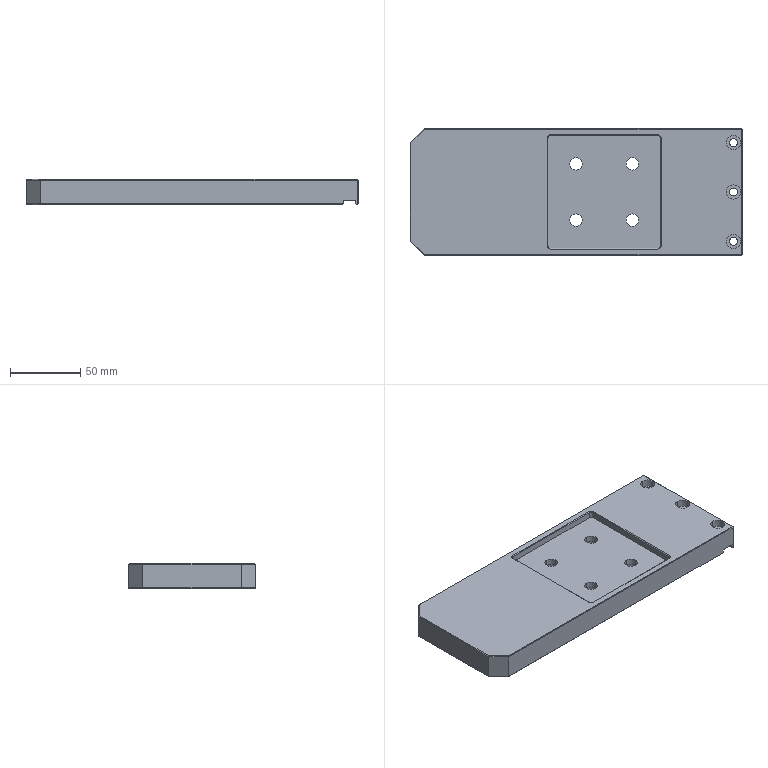NC program | NX | posted with a generic post | part box 235.5 x 90 x 18 mm
Whole program:
N10 G17 G21 G94 G90
(HOLE_MILLING_COPY , TOOL : D6)
N12 T06 M6
N14 G54
N16 G17 G0 G90 X0. Y20. S9500 M3
N18 G43 Z30. H6
N20 Z0.5
N22 G94 G3 X1.125 Y18.875 R1.125 F1500.
N24 X2.25 Y20. R1.125
N26 X2.25 Y20. Z-0.1 I-2.25 J0.
N28 X2.25 Y20. Z-0.7 I-2.25 J0.
N30 X2.25 Y20. Z-1.3 I-2.25 J0.
N32 X2.25 Y20. Z-1.9 I-2.25 J0.
N34 X2.25 Y20. Z-2.5 I-2.25 J0.
N36 X2.25 Y20. Z-3.1 I-2.25 J0.
N38 X2.25 Y20. Z-3.7 I-2.25 J0.
N40 X2.25 Y20. Z-4.3 I-2.25 J0.
N42 X2.25 Y20. Z-4.9 I-2.25 J0.
N44 X2.25 Y20. Z-5.5 I-2.25 J0.
N46 X2.25 Y20. Z-6.1 I-2.25 J0.
N48 X2.25 Y20. Z-6.7 I-2.25 J0.
N50 X2.25 Y20. Z-7.3 I-2.25 J0.
N52 X2.25 Y20. Z-7.9 I-2.25 J0.
N54 X2.25 Y20. Z-8.5 I-2.25 J0.
N56 X1.125 Y21.949 Z-8.6 R2.25
N58 X-1.949 Y21.125 R2.25
N60 X1.125 Y21.949 R-2.25
N62 X-0.412 Y21.537 R1.125
N64 X0. Y20. R1.125
N66 G0 Z0.5
N68 G3 X2.25 Y17.75 R2.25
N70 X4.5 Y20. R2.25
N72 X4.5 Y20. Z-0.1 I-4.5 J0.
N74 X4.5 Y20. Z-0.7 I-4.5 J0.
N76 X4.5 Y20. Z-1.3 I-4.5 J0.
N78 X4.5 Y20. Z-1.9 I-4.5 J0.
N80 X4.5 Y20. Z-2.5 I-4.5 J0.
N82 X4.5 Y20. Z-3.1 I-4.5 J0.
N84 X4.5 Y20. Z-3.7 I-4.5 J0.
N86 X4.5 Y20. Z-4.3 I-4.5 J0.
N88 X4.5 Y20. Z-4.9 I-4.5 J0.
N90 X4.5 Y20. Z-5.5 I-4.5 J0.
N92 X4.5 Y20. Z-6.1 I-4.5 J0.
N94 X4.5 Y20. Z-6.7 I-4.5 J0.
N96 X4.5 Y20. Z-7.3 I-4.5 J0.
N98 X4.5 Y20. Z-7.9 I-4.5 J0.
N100 X4.5 Y20. Z-8.5 I-4.5 J0.
N102 X2.25 Y23.897 Z-8.6 R4.5
N104 X-3.897 Y22.25 R4.5
N106 X2.25 Y23.897 R-4.5
N108 X-0.824 Y23.074 R2.25
N110 X0. Y20. R2.25
N112 G0 Z30.
N114 X40.
N116 Z0.5
N118 G3 X41.125 Y18.875 R1.125
N120 X42.25 Y20. R1.125
N122 X42.25 Y20. Z-0.1 I-2.25 J0.
N124 X42.25 Y20. Z-0.7 I-2.25 J0.
N126 X42.25 Y20. Z-1.3 I-2.25 J0.
N128 X42.25 Y20. Z-1.9 I-2.25 J0.
N130 X42.25 Y20. Z-2.5 I-2.25 J0.
N132 X42.25 Y20. Z-3.1 I-2.25 J0.
N134 X42.25 Y20. Z-3.7 I-2.25 J0.
N136 X42.25 Y20. Z-4.3 I-2.25 J0.
N138 X42.25 Y20. Z-4.9 I-2.25 J0.
N140 X42.25 Y20. Z-5.5 I-2.25 J0.
N142 X42.25 Y20. Z-6.1 I-2.25 J0.
N144 X42.25 Y20. Z-6.7 I-2.25 J0.
N146 X42.25 Y20. Z-7.3 I-2.25 J0.
N148 X42.25 Y20. Z-7.9 I-2.25 J0.
N150 X42.25 Y20. Z-8.5 I-2.25 J0.
N152 X41.125 Y21.949 Z-8.6 R2.25
N154 X38.051 Y21.125 R2.25
N156 X41.125 Y21.949 R-2.25
N158 X39.588 Y21.537 R1.125
N160 X40. Y20. R1.125
N162 G0 Z0.5
N164 G3 X42.25 Y17.75 R2.25
N166 X44.5 Y20. R2.25
N168 X44.5 Y20. Z-0.1 I-4.5 J0.
N170 X44.5 Y20. Z-0.7 I-4.5 J0.
N172 X44.5 Y20. Z-1.3 I-4.5 J0.
N174 X44.5 Y20. Z-1.9 I-4.5 J0.
N176 X44.5 Y20. Z-2.5 I-4.5 J0.
N178 X44.5 Y20. Z-3.1 I-4.5 J0.
N180 X44.5 Y20. Z-3.7 I-4.5 J0.
N182 X44.5 Y20. Z-4.3 I-4.5 J0.
N184 X44.5 Y20. Z-4.9 I-4.5 J0.
N186 X44.5 Y20. Z-5.5 I-4.5 J0.
N188 X44.5 Y20. Z-6.1 I-4.5 J0.
N190 X44.5 Y20. Z-6.7 I-4.5 J0.
N192 X44.5 Y20. Z-7.3 I-4.5 J0.
N194 X44.5 Y20. Z-7.9 I-4.5 J0.
N196 X44.5 Y20. Z-8.5 I-4.5 J0.
N198 X42.25 Y23.897 Z-8.6 R4.5
N200 X36.103 Y22.25 R4.5
N202 X42.25 Y23.897 R-4.5
N204 X39.176 Y23.074 R2.25
N206 X40. Y20. R2.25
N208 G0 Z30.
N210 Y-20.
N212 Z0.5
N214 G3 X41.125 Y-21.125 R1.125
N216 X42.25 Y-20. R1.125
N218 X42.25 Y-20. Z-0.1 I-2.25 J0.
N220 X42.25 Y-20. Z-0.7 I-2.25 J0.
N222 X42.25 Y-20. Z-1.3 I-2.25 J0.
N224 X42.25 Y-20. Z-1.9 I-2.25 J0.
N226 X42.25 Y-20. Z-2.5 I-2.25 J0.
N228 X42.25 Y-20. Z-3.1 I-2.25 J0.
N230 X42.25 Y-20. Z-3.7 I-2.25 J0.
N232 X42.25 Y-20. Z-4.3 I-2.25 J0.
N234 X42.25 Y-20. Z-4.9 I-2.25 J0.
N236 X42.25 Y-20. Z-5.5 I-2.25 J0.
N238 X42.25 Y-20. Z-6.1 I-2.25 J0.
N240 X42.25 Y-20. Z-6.7 I-2.25 J0.
N242 X42.25 Y-20. Z-7.3 I-2.25 J0.
N244 X42.25 Y-20. Z-7.9 I-2.25 J0.
N246 X42.25 Y-20. Z-8.5 I-2.25 J0.
N248 X41.125 Y-18.051 Z-8.6 R2.25
N250 X38.051 Y-18.875 R2.25
N252 X41.125 Y-18.051 R-2.25
N254 X39.588 Y-18.463 R1.125
N256 X40. Y-20. R1.125
N258 G0 Z0.5
N260 G3 X42.25 Y-22.25 R2.25
N262 X44.5 Y-20. R2.25
N264 X44.5 Y-20. Z-0.1 I-4.5 J0.
N266 X44.5 Y-20. Z-0.7 I-4.5 J0.
N268 X44.5 Y-20. Z-1.3 I-4.5 J0.
N270 X44.5 Y-20. Z-1.9 I-4.5 J0.
N272 X44.5 Y-20. Z-2.5 I-4.5 J0.
N274 X44.5 Y-20. Z-3.1 I-4.5 J0.
N276 X44.5 Y-20. Z-3.7 I-4.5 J0.
N278 X44.5 Y-20. Z-4.3 I-4.5 J0.
N280 X44.5 Y-20. Z-4.9 I-4.5 J0.
N282 X44.5 Y-20. Z-5.5 I-4.5 J0.
N284 X44.5 Y-20. Z-6.1 I-4.5 J0.
N286 X44.5 Y-20. Z-6.7 I-4.5 J0.
N288 X44.5 Y-20. Z-7.3 I-4.5 J0.
N290 X44.5 Y-20. Z-7.9 I-4.5 J0.
N292 X44.5 Y-20. Z-8.5 I-4.5 J0.
N294 X42.25 Y-16.103 Z-8.6 R4.5
N296 X36.103 Y-17.75 R4.5
N298 X42.25 Y-16.103 R-4.5
N300 X39.176 Y-16.926 R2.25
N302 X40. Y-20. R2.25
N304 G0 Z30.
N306 X0.
N308 Z0.5
N310 G3 X1.125 Y-21.125 R1.125
N312 X2.25 Y-20. R1.125
N314 X2.25 Y-20. Z-0.1 I-2.25 J0.
N316 X2.25 Y-20. Z-0.7 I-2.25 J0.
N318 X2.25 Y-20. Z-1.3 I-2.25 J0.
N320 X2.25 Y-20. Z-1.9 I-2.25 J0.
N322 X2.25 Y-20. Z-2.5 I-2.25 J0.
N324 X2.25 Y-20. Z-3.1 I-2.25 J0.
N326 X2.25 Y-20. Z-3.7 I-2.25 J0.
N328 X2.25 Y-20. Z-4.3 I-2.25 J0.
N330 X2.25 Y-20. Z-4.9 I-2.25 J0.
N332 X2.25 Y-20. Z-5.5 I-2.25 J0.
N334 X2.25 Y-20. Z-6.1 I-2.25 J0.
N336 X2.25 Y-20. Z-6.7 I-2.25 J0.
N338 X2.25 Y-20. Z-7.3 I-2.25 J0.
N340 X2.25 Y-20. Z-7.9 I-2.25 J0.
N342 X2.25 Y-20. Z-8.5 I-2.25 J0.
N344 X1.125 Y-18.051 Z-8.6 R2.25
N346 X-1.949 Y-18.875 R2.25
N348 X1.125 Y-18.051 R-2.25
N350 X-0.412 Y-18.463 R1.125
N352 X0. Y-20. R1.125
N354 G0 Z0.5
N356 G3 X2.25 Y-22.25 R2.25
N358 X4.5 Y-20. R2.25
N360 X4.5 Y-20. Z-0.1 I-4.5 J0.
N362 X4.5 Y-20. Z-0.7 I-4.5 J0.
N364 X4.5 Y-20. Z-1.3 I-4.5 J0.
N366 X4.5 Y-20. Z-1.9 I-4.5 J0.
N368 X4.5 Y-20. Z-2.5 I-4.5 J0.
N370 X4.5 Y-20. Z-3.1 I-4.5 J0.
N372 X4.5 Y-20. Z-3.7 I-4.5 J0.
N374 X4.5 Y-20. Z-4.3 I-4.5 J0.
N376 X4.5 Y-20. Z-4.9 I-4.5 J0.
N378 X4.5 Y-20. Z-5.5 I-4.5 J0.
N380 X4.5 Y-20. Z-6.1 I-4.5 J0.
N382 X4.5 Y-20. Z-6.7 I-4.5 J0.
N384 X4.5 Y-20. Z-7.3 I-4.5 J0.
N386 X4.5 Y-20. Z-7.9 I-4.5 J0.
N388 X4.5 Y-20. Z-8.5 I-4.5 J0.
N390 X2.25 Y-16.103 Z-8.6 R4.5
N392 X-3.897 Y-17.75 R4.5
N394 X2.25 Y-16.103 R-4.5
N396 X-0.824 Y-16.926 R2.25
N398 X0. Y-20. R2.25
N400 G0 Z30.
(FLOOR_WALL_COPY_1 , TOOL : D6)
N402 X112.731 Y-49.1
N404 Z0.758
N406 G1 Z-0.242 F1000.
N408 X112.27 Y-48.3
N410 G3 X111.75 Y-48. R0.6
N412 G1 X110.35 F3500.
N414 Y48.
N416 X113.15
N418 Y-48.
N420 X111.75
N422 G3 X111.23 Y-48.3 R0.6
N424 G1 X110.826 Y-49.
N426 Z0.758
N428 G0 Z3.
N430 X112.731 Y-49.1
N432 Z0.517
N434 G1 Z-0.483 F1000.
N436 X112.27 Y-48.3
N438 G3 X111.75 Y-48. R0.6
N440 G1 X110.35 F3500.
N442 Y48.
N444 X113.15
N446 Y-48.
N448 X111.75
N450 G3 X111.23 Y-48.3 R0.6
N452 G1 X110.778 Y-49.083
N454 Z0.517
N456 G0 Z2.758
N458 X112.731 Y-49.1
N460 Z0.275
N462 G1 Z-0.725 F1000.
N464 X112.27 Y-48.3
N466 G3 X111.75 Y-48. R0.6
N468 G1 X110.35 F3500.
N470 Y48.
N472 X113.15
N474 Y-48.
N476 X111.75
N478 G3 X111.23 Y-48.3 R0.6
N480 G1 X110.769 Y-49.1
N482 Z0.275
N484 G0 Z2.517
N486 X112.731
N488 Z0.033
N490 G1 Z-0.967 F1000.
N492 X112.27 Y-48.3
N494 G3 X111.75 Y-48. R0.6
N496 G1 X110.35 F3500.
N498 Y48.
N500 X113.15
N502 Y-48.
N504 X111.75
N506 G3 X111.23 Y-48.3 R0.6
N508 G1 X110.769 Y-49.1
N510 Z0.033
N512 G0 Z2.275
N514 X112.731
N516 Z-0.208
N518 G1 Z-1.208 F1000.
N520 X112.27 Y-48.3
N522 G3 X111.75 Y-48. R0.6
N524 G1 X110.35 F3500.
N526 Y48.
N528 X113.15
N530 Y-48.
N532 X111.75
N534 G3 X111.23 Y-48.3 R0.6
N536 G1 X110.769 Y-49.1
N538 Z-0.208
N540 G0 Z2.033
N542 X112.731
N544 Z-0.45
N546 G1 Z-1.45 F1000.
N548 X112.27 Y-48.3
N550 G3 X111.75 Y-48. R0.6
N552 G1 X110.35 F3500.
N554 Y48.
N556 X113.15
N558 Y-48.
N560 X111.75
N562 G3 X111.23 Y-48.3 R0.6
N564 G1 X110.769 Y-49.1
N566 Z-0.45
N568 G0 Z1.792
N570 X112.731
N572 Z-0.692
N574 G1 Z-1.692 F1000.
N576 X112.27 Y-48.3
N578 G3 X111.75 Y-48. R0.6
N580 G1 X110.35 F3500.
N582 Y48.
N584 X113.15
N586 Y-48.
N588 X111.75
N590 G3 X111.23 Y-48.3 R0.6
N592 G1 X110.769 Y-49.1
N594 Z-0.692
N596 G0 Z1.55
N598 X112.731
N600 Z-0.933
N602 G1 Z-1.933 F1000.
N604 X112.27 Y-48.3
N606 G3 X111.75 Y-48. R0.6
N608 G1 X110.35 F3500.
N610 Y48.
N612 X113.15
N614 Y-48.
N616 X111.75
N618 G3 X111.23 Y-48.3 R0.6
N620 G1 X110.769 Y-49.1
N622 Z-0.933
N624 G0 Z1.308
N626 X112.731
N628 Z-1.175
N630 G1 Z-2.175 F1000.
N632 X112.27 Y-48.3
N634 G3 X111.75 Y-48. R0.6
N636 G1 X110.35 F3500.
N638 Y48.
N640 X113.15
N642 Y-48.
N644 X111.75
N646 G3 X111.23 Y-48.3 R0.6
N648 G1 X110.769 Y-49.1
N650 Z-1.175
N652 G0 Z1.067
N654 X112.731
N656 Z-1.417
N658 G1 Z-2.417 F1000.
N660 X112.27 Y-48.3
N662 G3 X111.75 Y-48. R0.6
N664 G1 X110.35 F3500.
N666 Y48.
N668 X113.15
N670 Y-48.
N672 X111.75
N674 G3 X111.23 Y-48.3 R0.6
N676 G1 X110.769 Y-49.1
N678 Z-1.417
N680 G0 Z0.825
N682 X112.731
N684 Z-1.658
N686 G1 Z-2.658 F1000.
N688 X112.27 Y-48.3
N690 G3 X111.75 Y-48. R0.6
N692 G1 X110.35 F3500.
N694 Y48.
N696 X113.15
N698 Y-48.
N700 X111.75
N702 G3 X111.23 Y-48.3 R0.6
N704 G1 X110.769 Y-49.1
N706 Z-1.658
N708 G0 Z0.583
N710 X112.731
N712 Z-1.9
N714 G1 Z-2.9 F1000.
N716 X112.27 Y-48.3
N718 G3 X111.75 Y-48. R0.6
N720 G1 X110.35 F3500.
N722 Y48.
N724 X113.15
N726 Y-48.
N728 X111.75
N730 G3 X111.23 Y-48.3 R0.6
N732 G1 X110.769 Y-49.1
N734 Z-1.9
N736 G0 Z30.
(FLOOR_WALL_COPY_COPY , TOOL : D6)
N738 X110.826 Y-49.
N740 Z-2.
N742 G1 Z-3. F1000.
N744 X111.23 Y-48.3
N746 G2 X111.75 Y-48. R0.6
N748 G1 X112.95 F1500.
N750 Y48.
N752 X110.55
N754 Y-48.
N756 X111.75
N758 G2 X112.27 Y-48.3 R0.6
N760 G1 X112.674 Y-49.
N762 Z-2.
N764 G0 Z0.1
N766 X112.118
N768 Z-2.
N770 G1 Z-3. F1000.
N772 X112.95 Y-48.52
N774 G3 X113.25 Y-48. R0.6
N776 G1 Y48. F1500.
N778 G3 X112.95 Y48.52 R0.6
N780 G1 X110.55
N782 G3 X110.25 Y48. R0.6 F1000.
N784 G1 Y-48. F1500.
N786 G3 X110.55 Y-48.52 R0.6
N788 G1 X111.382 Y-49.
N790 Z-2.
N792 G0 Z30.
N794 M5
(PLANAR_MILL_COPY_1 , TOOL : D6A45)
N796 T01 M6
N798 G54
N800 G17 G0 G90 X39.031 Y-25.921 S9500 M3
N802 G43 Z30. H1
N804 Z0.
N806 G94 G1 Z-1. F1500.
N808 X39.134 Y-26.1
N810 G3 X40. Y-26.6 R1.
N812 X46.6 Y-20. R6.6
N814 X40. Y-26.6 R-6.6
N816 X40.866 Y-26.1 R1.
N818 G1 X40.969 Y-25.921
N820 Z0.
N822 G0 Z30.
N824 X39.031 Y14.079
N826 Z0.
N828 G1 Z-1.
N830 X39.134 Y13.9
N832 G3 X40. Y13.4 R1.
N834 X46.6 Y20. R6.6
N836 X40. Y13.4 R-6.6
N838 X40.866 Y13.9 R1.
N840 G1 X40.969 Y14.079
N842 Z0.
N844 G0 Z30.
N846 X-0.969
N848 Z0.
N850 G1 Z-1.
N852 X-0.866 Y13.9
N854 G3 X0. Y13.4 R1.
N856 X6.6 Y20. R6.6
N858 X0. Y13.4 R-6.6
N860 X0.866 Y13.9 R1.
N862 G1 X0.969 Y14.079
N864 Z0.
N866 G0 Z30.
N868 X-0.969 Y-25.921
N870 Z0.
N872 G1 Z-1.
N874 X-0.866 Y-26.1
N876 G3 X0. Y-26.6 R1.
N878 X6.6 Y-20. R6.6
N880 X0. Y-26.6 R-6.6
N882 X0.866 Y-26.1 R1.
N884 G1 X0.969 Y-25.921
N886 Z0.
N888 G0 Z30.
(PLANAR_MILL_COPY_1_COPY , TOOL : D6A45)
N890 X-1.32 Y46.1
N892 Z0.
N894 G1 Z-1.
N896 X-1.262 Y46.
N898 G3 X-0.396 Y45.5 R1.
N900 G1 X106.75
N902 G2 X107.75 Y44.5 R1.
N904 G1 Y-44.5
N906 G2 X106.75 Y-45.5 R1.
N908 G1 X-107.543
N910 G2 X-108.25 Y-45.207 R1.
N912 G1 X-117.957 Y-35.5
N914 G2 X-118.25 Y-34.793 R1.
N916 G1 Y34.793
N918 G2 X-117.957 Y35.5 R1.
N920 G1 X-108.25 Y45.207
N922 G2 X-107.543 Y45.5 R1.
N924 G1 X-0.396
N926 G3 X0.47 Y46. R1.
N928 G1 X0.527 Y46.1
N930 Z0.
N932 G0 Z30.
(PLANAR_MILL_COPY_1_COPY_COPY , TOOL : D6A45)
N934 X115.36 Y-45.792
N936 Z0.
N938 G1 Z-1. F1000.
N940 G3 X115.75 Y-45. R1.
N942 G1 Y45.
N944 G2 X116.75 Y46. R1.
N946 G1 X117.25
N948 G2 X118.25 Y45. R1.
N950 G1 Y-45.
N952 G2 X117.25 Y-46. R1.
N954 G1 X116.75
N956 G2 X115.75 Y-45. R1.
N958 G3 X115.25 Y-44.134 R1.
N960 G1 X115.15 Y-44.076
N962 Z0.
N964 G0 Z30.
N966 M5
N968 M2